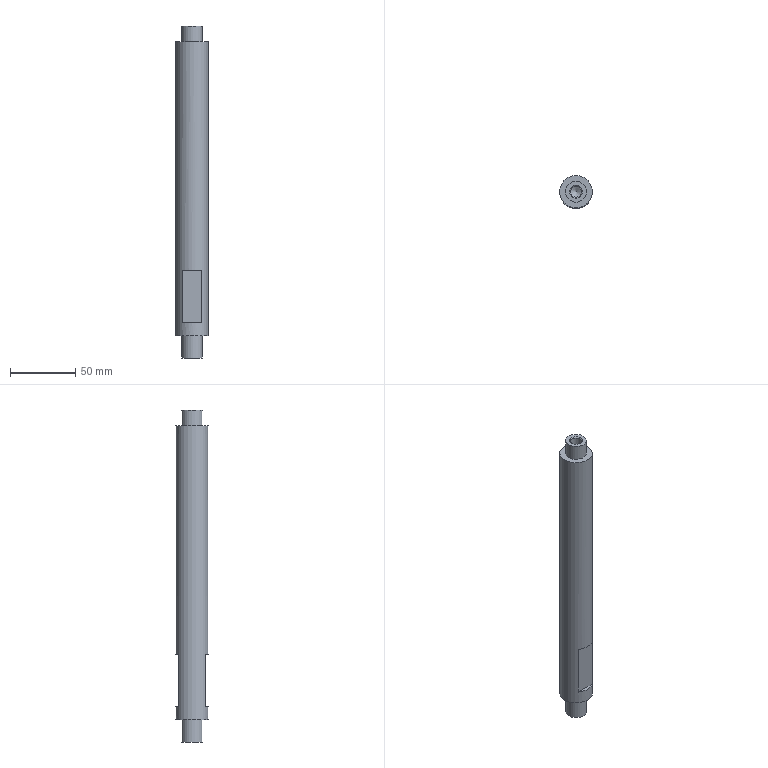Part | STEP file | YBQDJ-QD-2 | 1 solid | 19 faces | box 25 x 25 x 254 mm | volume 111454 mm3 | plane 10 | cylinder 5 | cone 4 | commonest cylinder face diameters 8.5 x2 16 x2 25 x1
STEP:
#1=CARTESIAN_POINT('',(0.,0.,0.));
#2=DIRECTION('',(0.,0.,1.));
#3=DIRECTION('',(1.,0.,0.));
#4=AXIS2_PLACEMENT_3D('',#1,#2,#3);
#5=CARTESIAN_POINT('',(-327.5,-310.,250.));
#6=VERTEX_POINT('',#5);
#7=CARTESIAN_POINT('',(-340.,-310.,250.));
#8=DIRECTION('',(0.,0.,1.));
#9=DIRECTION('',(1.,0.,0.));
#10=AXIS2_PLACEMENT_3D('',#7,#8,#9);
#11=CIRCLE('',#10,12.5);
#12=CARTESIAN_POINT('',(-340.,-310.,270.));
#13=DIRECTION('',(0.,0.,-1.));
#14=DIRECTION('',(-1.,0.,0.));
#15=AXIS2_PLACEMENT_3D('',#12,#13,#14);
#16=CYLINDRICAL_SURFACE('',#15,12.5);
#17=CARTESIAN_POINT('',(9.425,20.));
#18=DIRECTION('',(-1.,0.));
#19=VECTOR('',#18,1.);
#20=LINE('',#17,#19);
#21=(GEOMETRIC_REPRESENTATION_CONTEXT(2)PARAMETRIC_REPRESENTATION_CONTEXT()REPRESENTATION_CONTEXT('',''));
#22=DEFINITIONAL_REPRESENTATION('',(#20),#21);
#23=PCURVE('',#16,#22);
#24=CARTESIAN_POINT('',(-340.,-310.,250.));
#25=DIRECTION('',(0.,0.,1.));
#26=DIRECTION('',(1.,0.,0.));
#27=AXIS2_PLACEMENT_3D('',#24,#25,#26);
#28=PLANE('',#27);
#29=CARTESIAN_POINT('',(0.,0.));
#30=DIRECTION('',(1.,0.));
#31=AXIS2_PLACEMENT_2D('',#29,#30);
#32=CIRCLE('',#31,12.5);
#33=(GEOMETRIC_REPRESENTATION_CONTEXT(2)PARAMETRIC_REPRESENTATION_CONTEXT()REPRESENTATION_CONTEXT('',''));
#34=DEFINITIONAL_REPRESENTATION('',(#32),#33);
#35=PCURVE('',#28,#34);
#36=SURFACE_CURVE('',#11,(#23,#35),.PCURVE_S1.);
#37=EDGE_CURVE('',#6,#6,#36,.T.);
#38=ORIENTED_EDGE('',*,*,#37,.F.);
#39=CARTESIAN_POINT('',(-327.5,-310.,25.));
#40=VERTEX_POINT('',#39);
#41=CARTESIAN_POINT('',(-327.5,-310.,250.));
#42=CARTESIAN_POINT('',(-327.5,-310.,25.));
#43=B_SPLINE_CURVE_WITH_KNOTS('',1,(#41,#42),.UNSPECIFIED.,.F.,.F.,(2,2),(20.,245.),.PIECEWISE_BEZIER_KNOTS.);
#44=CARTESIAN_POINT('',(9.425,0.));
#45=DIRECTION('',(0.,1.));
#46=VECTOR('',#45,1.);
#47=LINE('',#44,#46);
#48=(GEOMETRIC_REPRESENTATION_CONTEXT(2)PARAMETRIC_REPRESENTATION_CONTEXT()REPRESENTATION_CONTEXT('',''));
#49=DEFINITIONAL_REPRESENTATION('',(#47),#48);
#50=PCURVE('',#16,#49);
#51=CARTESIAN_POINT('',(3.142,0.));
#52=DIRECTION('',(0.,1.));
#53=VECTOR('',#52,1.);
#54=LINE('',#51,#53);
#55=(GEOMETRIC_REPRESENTATION_CONTEXT(2)PARAMETRIC_REPRESENTATION_CONTEXT()REPRESENTATION_CONTEXT('',''));
#56=DEFINITIONAL_REPRESENTATION('',(#54),#55);
#57=PCURVE('',#16,#56);
#58=SEAM_CURVE('',#43,(#50,#57),.PCURVE_S1.);
#59=EDGE_CURVE('',#6,#40,#58,.T.);
#60=ORIENTED_EDGE('',*,*,#59,.T.);
#61=CARTESIAN_POINT('',(-340.,-310.,25.));
#62=DIRECTION('',(0.,0.,1.));
#63=DIRECTION('',(1.,0.,0.));
#64=AXIS2_PLACEMENT_3D('',#61,#62,#63);
#65=CIRCLE('',#64,12.5);
#66=CARTESIAN_POINT('',(9.425,245.));
#67=DIRECTION('',(-1.,0.));
#68=VECTOR('',#67,1.);
#69=LINE('',#66,#68);
#70=(GEOMETRIC_REPRESENTATION_CONTEXT(2)PARAMETRIC_REPRESENTATION_CONTEXT()REPRESENTATION_CONTEXT('',''));
#71=DEFINITIONAL_REPRESENTATION('',(#69),#70);
#72=PCURVE('',#16,#71);
#73=CARTESIAN_POINT('',(92.5,10.,25.));
#74=DIRECTION('',(0.,0.,1.));
#75=DIRECTION('',(1.,0.,0.));
#76=AXIS2_PLACEMENT_3D('',#73,#74,#75);
#77=PLANE('',#76);
#78=CARTESIAN_POINT('',(-432.5,-320.));
#79=DIRECTION('',(1.,0.));
#80=AXIS2_PLACEMENT_2D('',#78,#79);
#81=CIRCLE('',#80,12.5);
#82=(GEOMETRIC_REPRESENTATION_CONTEXT(2)PARAMETRIC_REPRESENTATION_CONTEXT()REPRESENTATION_CONTEXT('',''));
#83=DEFINITIONAL_REPRESENTATION('',(#81),#82);
#84=PCURVE('',#77,#83);
#85=SURFACE_CURVE('',#65,(#72,#84),.PCURVE_S1.);
#86=EDGE_CURVE('',#40,#40,#85,.T.);
#87=ORIENTED_EDGE('',*,*,#86,.T.);
#88=ORIENTED_EDGE('',*,*,#59,.F.);
#89=EDGE_LOOP('',(#38,#60,#87,#88));
#90=FACE_BOUND('',#89,.T.);
#91=CARTESIAN_POINT('',(-347.5,-300.,75.));
#92=VERTEX_POINT('',#91);
#93=CARTESIAN_POINT('',(-332.5,-300.,75.));
#94=VERTEX_POINT('',#93);
#95=CARTESIAN_POINT('',(-340.,-310.,75.));
#96=DIRECTION('',(0.,0.,-1.));
#97=DIRECTION('',(0.,1.,0.));
#98=AXIS2_PLACEMENT_3D('',#95,#96,#97);
#99=CIRCLE('',#98,12.5);
#100=CARTESIAN_POINT('',(1.571,195.));
#101=DIRECTION('',(1.,0.));
#102=VECTOR('',#101,1.);
#103=LINE('',#100,#102);
#104=(GEOMETRIC_REPRESENTATION_CONTEXT(2)PARAMETRIC_REPRESENTATION_CONTEXT()REPRESENTATION_CONTEXT('',''));
#105=DEFINITIONAL_REPRESENTATION('',(#103),#104);
#106=PCURVE('',#16,#105);
#107=CARTESIAN_POINT('',(-382.,-300.,75.));
#108=DIRECTION('',(0.,0.,-1.));
#109=DIRECTION('',(0.,1.,0.));
#110=AXIS2_PLACEMENT_3D('',#107,#108,#109);
#111=PLANE('',#110);
#112=CARTESIAN_POINT('',(-10.,42.));
#113=DIRECTION('',(1.,0.));
#114=AXIS2_PLACEMENT_2D('',#112,#113);
#115=CIRCLE('',#114,12.5);
#116=(GEOMETRIC_REPRESENTATION_CONTEXT(2)PARAMETRIC_REPRESENTATION_CONTEXT()REPRESENTATION_CONTEXT('',''));
#117=DEFINITIONAL_REPRESENTATION('',(#115),#116);
#118=PCURVE('',#111,#117);
#119=SURFACE_CURVE('',#99,(#106,#118),.PCURVE_S1.);
#120=EDGE_CURVE('',#92,#94,#119,.T.);
#121=ORIENTED_EDGE('',*,*,#120,.F.);
#122=CARTESIAN_POINT('',(-347.5,-300.,35.));
#123=VERTEX_POINT('',#122);
#124=CARTESIAN_POINT('',(-347.5,-300.,270.));
#125=DIRECTION('',(0.,0.,1.));
#126=VECTOR('',#125,1.);
#127=LINE('',#124,#126);
#128=CARTESIAN_POINT('',(7.21,0.));
#129=DIRECTION('',(0.,-1.));
#130=VECTOR('',#129,1.);
#131=LINE('',#128,#130);
#132=(GEOMETRIC_REPRESENTATION_CONTEXT(2)PARAMETRIC_REPRESENTATION_CONTEXT()REPRESENTATION_CONTEXT('',''));
#133=DEFINITIONAL_REPRESENTATION('',(#131),#132);
#134=PCURVE('',#16,#133);
#135=CARTESIAN_POINT('',(-382.,-300.,35.));
#136=DIRECTION('',(0.,1.,0.));
#137=DIRECTION('',(0.,0.,1.));
#138=AXIS2_PLACEMENT_3D('',#135,#136,#137);
#139=PLANE('',#138);
#140=CARTESIAN_POINT('',(235.,34.5));
#141=DIRECTION('',(1.,0.));
#142=VECTOR('',#141,1.);
#143=LINE('',#140,#142);
#144=(GEOMETRIC_REPRESENTATION_CONTEXT(2)PARAMETRIC_REPRESENTATION_CONTEXT()REPRESENTATION_CONTEXT('',''));
#145=DEFINITIONAL_REPRESENTATION('',(#143),#144);
#146=PCURVE('',#139,#145);
#147=SURFACE_CURVE('',#127,(#134,#146),.PCURVE_S1.);
#148=EDGE_CURVE('',#123,#92,#147,.T.);
#149=ORIENTED_EDGE('',*,*,#148,.F.);
#150=CARTESIAN_POINT('',(-332.5,-300.,35.));
#151=VERTEX_POINT('',#150);
#152=CARTESIAN_POINT('',(-340.,-310.,35.));
#153=DIRECTION('',(0.,0.,1.));
#154=DIRECTION('',(0.,-1.,0.));
#155=AXIS2_PLACEMENT_3D('',#152,#153,#154);
#156=CIRCLE('',#155,12.5);
#157=CARTESIAN_POINT('',(10.996,235.));
#158=DIRECTION('',(-1.,0.));
#159=VECTOR('',#158,1.);
#160=LINE('',#157,#159);
#161=(GEOMETRIC_REPRESENTATION_CONTEXT(2)PARAMETRIC_REPRESENTATION_CONTEXT()REPRESENTATION_CONTEXT('',''));
#162=DEFINITIONAL_REPRESENTATION('',(#160),#161);
#163=PCURVE('',#16,#162);
#164=CARTESIAN_POINT('',(-382.,-281.,35.));
#165=DIRECTION('',(0.,0.,1.));
#166=DIRECTION('',(0.,-1.,0.));
#167=AXIS2_PLACEMENT_3D('',#164,#165,#166);
#168=PLANE('',#167);
#169=CARTESIAN_POINT('',(29.,42.));
#170=DIRECTION('',(1.,0.));
#171=AXIS2_PLACEMENT_2D('',#169,#170);
#172=CIRCLE('',#171,12.5);
#173=(GEOMETRIC_REPRESENTATION_CONTEXT(2)PARAMETRIC_REPRESENTATION_CONTEXT()REPRESENTATION_CONTEXT('',''));
#174=DEFINITIONAL_REPRESENTATION('',(#172),#173);
#175=PCURVE('',#168,#174);
#176=SURFACE_CURVE('',#156,(#163,#175),.PCURVE_S1.);
#177=EDGE_CURVE('',#151,#123,#176,.T.);
#178=ORIENTED_EDGE('',*,*,#177,.F.);
#179=CARTESIAN_POINT('',(-332.5,-300.,270.));
#180=DIRECTION('',(0.,0.,-1.));
#181=VECTOR('',#180,1.);
#182=LINE('',#179,#181);
#183=CARTESIAN_POINT('',(8.497,0.));
#184=DIRECTION('',(0.,1.));
#185=VECTOR('',#184,1.);
#186=LINE('',#183,#185);
#187=(GEOMETRIC_REPRESENTATION_CONTEXT(2)PARAMETRIC_REPRESENTATION_CONTEXT()REPRESENTATION_CONTEXT('',''));
#188=DEFINITIONAL_REPRESENTATION('',(#186),#187);
#189=PCURVE('',#16,#188);
#190=CARTESIAN_POINT('',(235.,49.5));
#191=DIRECTION('',(-1.,0.));
#192=VECTOR('',#191,1.);
#193=LINE('',#190,#192);
#194=(GEOMETRIC_REPRESENTATION_CONTEXT(2)PARAMETRIC_REPRESENTATION_CONTEXT()REPRESENTATION_CONTEXT('',''));
#195=DEFINITIONAL_REPRESENTATION('',(#193),#194);
#196=PCURVE('',#139,#195);
#197=SURFACE_CURVE('',#182,(#189,#196),.PCURVE_S1.);
#198=EDGE_CURVE('',#94,#151,#197,.T.);
#199=ORIENTED_EDGE('',*,*,#198,.F.);
#200=EDGE_LOOP('',(#121,#149,#178,#199));
#201=FACE_BOUND('',#200,.T.);
#202=CARTESIAN_POINT('',(-332.5,-320.,75.));
#203=VERTEX_POINT('',#202);
#204=CARTESIAN_POINT('',(-347.5,-320.,75.));
#205=VERTEX_POINT('',#204);
#206=CARTESIAN_POINT('',(-340.,-310.,75.));
#207=DIRECTION('',(0.,0.,-1.));
#208=DIRECTION('',(0.,1.,0.));
#209=AXIS2_PLACEMENT_3D('',#206,#207,#208);
#210=CIRCLE('',#209,12.5);
#211=CARTESIAN_POINT('',(1.571,195.));
#212=DIRECTION('',(1.,0.));
#213=VECTOR('',#212,1.);
#214=LINE('',#211,#213);
#215=(GEOMETRIC_REPRESENTATION_CONTEXT(2)PARAMETRIC_REPRESENTATION_CONTEXT()REPRESENTATION_CONTEXT('',''));
#216=DEFINITIONAL_REPRESENTATION('',(#214),#215);
#217=PCURVE('',#16,#216);
#218=CARTESIAN_POINT('',(-382.,-339.,75.));
#219=DIRECTION('',(0.,0.,-1.));
#220=DIRECTION('',(0.,1.,0.));
#221=AXIS2_PLACEMENT_3D('',#218,#219,#220);
#222=PLANE('',#221);
#223=CARTESIAN_POINT('',(29.,42.));
#224=DIRECTION('',(1.,0.));
#225=AXIS2_PLACEMENT_2D('',#223,#224);
#226=CIRCLE('',#225,12.5);
#227=(GEOMETRIC_REPRESENTATION_CONTEXT(2)PARAMETRIC_REPRESENTATION_CONTEXT()REPRESENTATION_CONTEXT('',''));
#228=DEFINITIONAL_REPRESENTATION('',(#226),#227);
#229=PCURVE('',#222,#228);
#230=SURFACE_CURVE('',#210,(#217,#229),.PCURVE_S1.);
#231=EDGE_CURVE('',#203,#205,#230,.T.);
#232=ORIENTED_EDGE('',*,*,#231,.F.);
#233=CARTESIAN_POINT('',(-332.5,-320.,35.));
#234=VERTEX_POINT('',#233);
#235=CARTESIAN_POINT('',(-332.5,-320.,270.));
#236=DIRECTION('',(0.,0.,1.));
#237=VECTOR('',#236,1.);
#238=LINE('',#235,#237);
#239=CARTESIAN_POINT('',(4.069,0.));
#240=DIRECTION('',(0.,-1.));
#241=VECTOR('',#240,1.);
#242=LINE('',#239,#241);
#243=(GEOMETRIC_REPRESENTATION_CONTEXT(2)PARAMETRIC_REPRESENTATION_CONTEXT()REPRESENTATION_CONTEXT('',''));
#244=DEFINITIONAL_REPRESENTATION('',(#242),#243);
#245=PCURVE('',#16,#244);
#246=CARTESIAN_POINT('',(-382.,-320.,65.));
#247=DIRECTION('',(0.,-1.,0.));
#248=DIRECTION('',(0.,0.,-1.));
#249=AXIS2_PLACEMENT_3D('',#246,#247,#248);
#250=PLANE('',#249);
#251=CARTESIAN_POINT('',(-205.,49.5));
#252=DIRECTION('',(-1.,0.));
#253=VECTOR('',#252,1.);
#254=LINE('',#251,#253);
#255=(GEOMETRIC_REPRESENTATION_CONTEXT(2)PARAMETRIC_REPRESENTATION_CONTEXT()REPRESENTATION_CONTEXT('',''));
#256=DEFINITIONAL_REPRESENTATION('',(#254),#255);
#257=PCURVE('',#250,#256);
#258=SURFACE_CURVE('',#238,(#245,#257),.PCURVE_S1.);
#259=EDGE_CURVE('',#234,#203,#258,.T.);
#260=ORIENTED_EDGE('',*,*,#259,.F.);
#261=CARTESIAN_POINT('',(-347.5,-320.,35.));
#262=VERTEX_POINT('',#261);
#263=CARTESIAN_POINT('',(-340.,-310.,35.));
#264=DIRECTION('',(0.,0.,1.));
#265=DIRECTION('',(0.,-1.,0.));
#266=AXIS2_PLACEMENT_3D('',#263,#264,#265);
#267=CIRCLE('',#266,12.5);
#268=CARTESIAN_POINT('',(10.996,235.));
#269=DIRECTION('',(-1.,0.));
#270=VECTOR('',#269,1.);
#271=LINE('',#268,#270);
#272=(GEOMETRIC_REPRESENTATION_CONTEXT(2)PARAMETRIC_REPRESENTATION_CONTEXT()REPRESENTATION_CONTEXT('',''));
#273=DEFINITIONAL_REPRESENTATION('',(#271),#272);
#274=PCURVE('',#16,#273);
#275=CARTESIAN_POINT('',(-382.,-320.,35.));
#276=DIRECTION('',(0.,0.,1.));
#277=DIRECTION('',(0.,-1.,0.));
#278=AXIS2_PLACEMENT_3D('',#275,#276,#277);
#279=PLANE('',#278);
#280=CARTESIAN_POINT('',(-10.,42.));
#281=DIRECTION('',(1.,0.));
#282=AXIS2_PLACEMENT_2D('',#280,#281);
#283=CIRCLE('',#282,12.5);
#284=(GEOMETRIC_REPRESENTATION_CONTEXT(2)PARAMETRIC_REPRESENTATION_CONTEXT()REPRESENTATION_CONTEXT('',''));
#285=DEFINITIONAL_REPRESENTATION('',(#283),#284);
#286=PCURVE('',#279,#285);
#287=SURFACE_CURVE('',#267,(#274,#286),.PCURVE_S1.);
#288=EDGE_CURVE('',#262,#234,#287,.T.);
#289=ORIENTED_EDGE('',*,*,#288,.F.);
#290=CARTESIAN_POINT('',(-347.5,-320.,270.));
#291=DIRECTION('',(0.,0.,-1.));
#292=VECTOR('',#291,1.);
#293=LINE('',#290,#292);
#294=CARTESIAN_POINT('',(5.356,0.));
#295=DIRECTION('',(0.,1.));
#296=VECTOR('',#295,1.);
#297=LINE('',#294,#296);
#298=(GEOMETRIC_REPRESENTATION_CONTEXT(2)PARAMETRIC_REPRESENTATION_CONTEXT()REPRESENTATION_CONTEXT('',''));
#299=DEFINITIONAL_REPRESENTATION('',(#297),#298);
#300=PCURVE('',#16,#299);
#301=CARTESIAN_POINT('',(-205.,34.5));
#302=DIRECTION('',(1.,0.));
#303=VECTOR('',#302,1.);
#304=LINE('',#301,#303);
#305=(GEOMETRIC_REPRESENTATION_CONTEXT(2)PARAMETRIC_REPRESENTATION_CONTEXT()REPRESENTATION_CONTEXT('',''));
#306=DEFINITIONAL_REPRESENTATION('',(#304),#305);
#307=PCURVE('',#250,#306);
#308=SURFACE_CURVE('',#293,(#300,#307),.PCURVE_S1.);
#309=EDGE_CURVE('',#205,#262,#308,.T.);
#310=ORIENTED_EDGE('',*,*,#309,.F.);
#311=EDGE_LOOP('',(#232,#260,#289,#310));
#312=FACE_BOUND('',#311,.T.);
#313=ADVANCED_FACE('',(#90,#201,#312),#16,.T.);
#314=CARTESIAN_POINT('',(-332.,-310.,250.));
#315=VERTEX_POINT('',#314);
#316=CARTESIAN_POINT('',(-340.,-310.,250.));
#317=DIRECTION('',(0.,0.,1.));
#318=DIRECTION('',(1.,0.,0.));
#319=AXIS2_PLACEMENT_3D('',#316,#317,#318);
#320=CIRCLE('',#319,8.);
#321=CARTESIAN_POINT('',(0.,0.));
#322=DIRECTION('',(1.,0.));
#323=AXIS2_PLACEMENT_2D('',#321,#322);
#324=CIRCLE('',#323,8.);
#325=(GEOMETRIC_REPRESENTATION_CONTEXT(2)PARAMETRIC_REPRESENTATION_CONTEXT()REPRESENTATION_CONTEXT('',''));
#326=DEFINITIONAL_REPRESENTATION('',(#324),#325);
#327=PCURVE('',#28,#326);
#328=CARTESIAN_POINT('',(-340.,-310.,265.));
#329=DIRECTION('',(0.,0.,-1.));
#330=DIRECTION('',(-1.,0.,0.));
#331=AXIS2_PLACEMENT_3D('',#328,#329,#330);
#332=CYLINDRICAL_SURFACE('',#331,8.);
#333=CARTESIAN_POINT('',(9.425,15.));
#334=DIRECTION('',(-1.,0.));
#335=VECTOR('',#334,1.);
#336=LINE('',#333,#335);
#337=(GEOMETRIC_REPRESENTATION_CONTEXT(2)PARAMETRIC_REPRESENTATION_CONTEXT()REPRESENTATION_CONTEXT('',''));
#338=DEFINITIONAL_REPRESENTATION('',(#336),#337);
#339=PCURVE('',#332,#338);
#340=SURFACE_CURVE('',#320,(#327,#339),.PCURVE_S1.);
#341=EDGE_CURVE('',#315,#315,#340,.T.);
#342=ORIENTED_EDGE('',*,*,#341,.F.);
#343=EDGE_LOOP('',(#342));
#344=FACE_BOUND('',#343,.T.);
#345=ORIENTED_EDGE('',*,*,#37,.T.);
#346=EDGE_LOOP('',(#345));
#347=FACE_BOUND('',#346,.T.);
#348=ADVANCED_FACE('',(#344,#347),#28,.T.);
#349=CARTESIAN_POINT('',(-332.,-310.,25.));
#350=VERTEX_POINT('',#349);
#351=CARTESIAN_POINT('',(-340.,-310.,25.));
#352=DIRECTION('',(0.,0.,-1.));
#353=DIRECTION('',(1.,0.,0.));
#354=AXIS2_PLACEMENT_3D('',#351,#352,#353);
#355=CIRCLE('',#354,8.);
#356=CARTESIAN_POINT('',(-424.5,-320.));
#357=CARTESIAN_POINT('',(-424.5,-333.856));
#358=CARTESIAN_POINT('',(-436.5,-326.928));
#359=CARTESIAN_POINT('',(-448.5,-320.));
#360=CARTESIAN_POINT('',(-436.5,-313.072));
#361=CARTESIAN_POINT('',(-424.5,-306.144));
#362=CARTESIAN_POINT('',(-424.5,-320.));
#363=(BOUNDED_CURVE()B_SPLINE_CURVE(2,(#356,#357,#358,#359,#360,#361,#362),.UNSPECIFIED.,.T.,.F.)B_SPLINE_CURVE_WITH_KNOTS((1,2,2,2,2,1),(-2.094,0.,2.094,4.189,6.283,8.378),.UNSPECIFIED.)CURVE()GEOMETRIC_REPRESENTATION_ITEM()RATIONAL_B_SPLINE_CURVE((1.,0.5,1.,0.5,1.,0.5,1.))REPRESENTATION_ITEM(''));
#364=(GEOMETRIC_REPRESENTATION_CONTEXT(2)PARAMETRIC_REPRESENTATION_CONTEXT()REPRESENTATION_CONTEXT('',''));
#365=DEFINITIONAL_REPRESENTATION('',(#363),#364);
#366=PCURVE('',#77,#365);
#367=CARTESIAN_POINT('',(-340.,-310.,8.));
#368=DIRECTION('',(0.,0.,1.));
#369=DIRECTION('',(1.,0.,0.));
#370=AXIS2_PLACEMENT_3D('',#367,#368,#369);
#371=CYLINDRICAL_SURFACE('',#370,8.);
#372=CARTESIAN_POINT('',(6.283,17.));
#373=DIRECTION('',(-1.,0.));
#374=VECTOR('',#373,1.);
#375=LINE('',#372,#374);
#376=(GEOMETRIC_REPRESENTATION_CONTEXT(2)PARAMETRIC_REPRESENTATION_CONTEXT()REPRESENTATION_CONTEXT('',''));
#377=DEFINITIONAL_REPRESENTATION('',(#375),#376);
#378=PCURVE('',#371,#377);
#379=SURFACE_CURVE('',#355,(#366,#378),.PCURVE_S1.);
#380=EDGE_CURVE('',#350,#350,#379,.T.);
#381=ORIENTED_EDGE('',*,*,#380,.F.);
#382=EDGE_LOOP('',(#381));
#383=FACE_BOUND('',#382,.T.);
#384=ORIENTED_EDGE('',*,*,#86,.F.);
#385=EDGE_LOOP('',(#384));
#386=FACE_BOUND('',#385,.T.);
#387=ADVANCED_FACE('',(#383,#386),#77,.F.);
#388=CARTESIAN_POINT('',(-332.,-310.,262.));
#389=VERTEX_POINT('',#388);
#390=CARTESIAN_POINT('',(-340.,-310.,262.));
#391=DIRECTION('',(0.,0.,1.));
#392=DIRECTION('',(1.,0.,0.));
#393=AXIS2_PLACEMENT_3D('',#390,#391,#392);
#394=CIRCLE('',#393,8.);
#395=CARTESIAN_POINT('',(9.425,3.));
#396=DIRECTION('',(-1.,0.));
#397=VECTOR('',#396,1.);
#398=LINE('',#395,#397);
#399=(GEOMETRIC_REPRESENTATION_CONTEXT(2)PARAMETRIC_REPRESENTATION_CONTEXT()REPRESENTATION_CONTEXT('',''));
#400=DEFINITIONAL_REPRESENTATION('',(#398),#399);
#401=PCURVE('',#332,#400);
#402=CARTESIAN_POINT('',(-340.,-310.,262.));
#403=DIRECTION('',(0.,0.,1.));
#404=DIRECTION('',(1.,0.,0.));
#405=AXIS2_PLACEMENT_3D('',#402,#403,#404);
#406=PLANE('',#405);
#407=CARTESIAN_POINT('',(0.,0.));
#408=DIRECTION('',(1.,0.));
#409=AXIS2_PLACEMENT_2D('',#407,#408);
#410=CIRCLE('',#409,8.);
#411=(GEOMETRIC_REPRESENTATION_CONTEXT(2)PARAMETRIC_REPRESENTATION_CONTEXT()REPRESENTATION_CONTEXT('',''));
#412=DEFINITIONAL_REPRESENTATION('',(#410),#411);
#413=PCURVE('',#406,#412);
#414=SURFACE_CURVE('',#394,(#401,#413),.PCURVE_S1.);
#415=EDGE_CURVE('',#389,#389,#414,.T.);
#416=ORIENTED_EDGE('',*,*,#415,.F.);
#417=CARTESIAN_POINT('',(-332.,-310.,262.));
#418=CARTESIAN_POINT('',(-332.,-310.,250.));
#419=B_SPLINE_CURVE_WITH_KNOTS('',1,(#417,#418),.UNSPECIFIED.,.F.,.F.,(2,2),(3.,15.),.PIECEWISE_BEZIER_KNOTS.);
#420=CARTESIAN_POINT('',(9.425,0.));
#421=DIRECTION('',(0.,1.));
#422=VECTOR('',#421,1.);
#423=LINE('',#420,#422);
#424=(GEOMETRIC_REPRESENTATION_CONTEXT(2)PARAMETRIC_REPRESENTATION_CONTEXT()REPRESENTATION_CONTEXT('',''));
#425=DEFINITIONAL_REPRESENTATION('',(#423),#424);
#426=PCURVE('',#332,#425);
#427=CARTESIAN_POINT('',(3.142,0.));
#428=DIRECTION('',(0.,1.));
#429=VECTOR('',#428,1.);
#430=LINE('',#427,#429);
#431=(GEOMETRIC_REPRESENTATION_CONTEXT(2)PARAMETRIC_REPRESENTATION_CONTEXT()REPRESENTATION_CONTEXT('',''));
#432=DEFINITIONAL_REPRESENTATION('',(#430),#431);
#433=PCURVE('',#332,#432);
#434=SEAM_CURVE('',#419,(#426,#433),.PCURVE_S1.);
#435=EDGE_CURVE('',#389,#315,#434,.T.);
#436=ORIENTED_EDGE('',*,*,#435,.T.);
#437=ORIENTED_EDGE('',*,*,#341,.T.);
#438=ORIENTED_EDGE('',*,*,#435,.F.);
#439=EDGE_LOOP('',(#416,#436,#437,#438));
#440=FACE_BOUND('',#439,.T.);
#441=ADVANCED_FACE('',(#440),#332,.T.);
#442=CARTESIAN_POINT('',(-335.,-310.,262.));
#443=VERTEX_POINT('',#442);
#444=CARTESIAN_POINT('',(-340.,-310.,262.));
#445=DIRECTION('',(0.,0.,-1.));
#446=DIRECTION('',(1.,0.,0.));
#447=AXIS2_PLACEMENT_3D('',#444,#445,#446);
#448=CIRCLE('',#447,5.);
#449=CARTESIAN_POINT('',(5.,0.));
#450=CARTESIAN_POINT('',(5.,-8.66));
#451=CARTESIAN_POINT('',(-2.5,-4.33));
#452=CARTESIAN_POINT('',(-10.,0.));
#453=CARTESIAN_POINT('',(-2.5,4.33));
#454=CARTESIAN_POINT('',(5.,8.66));
#455=CARTESIAN_POINT('',(5.,0.));
#456=(BOUNDED_CURVE()B_SPLINE_CURVE(2,(#449,#450,#451,#452,#453,#454,#455),.UNSPECIFIED.,.T.,.F.)B_SPLINE_CURVE_WITH_KNOTS((1,2,2,2,2,1),(-2.094,0.,2.094,4.189,6.283,8.378),.UNSPECIFIED.)CURVE()GEOMETRIC_REPRESENTATION_ITEM()RATIONAL_B_SPLINE_CURVE((1.,0.5,1.,0.5,1.,0.5,1.))REPRESENTATION_ITEM(''));
#457=(GEOMETRIC_REPRESENTATION_CONTEXT(2)PARAMETRIC_REPRESENTATION_CONTEXT()REPRESENTATION_CONTEXT('',''));
#458=DEFINITIONAL_REPRESENTATION('',(#456),#457);
#459=PCURVE('',#406,#458);
#460=CARTESIAN_POINT('',(-340.,-310.,262.));
#461=DIRECTION('',(0.,0.,1.));
#462=DIRECTION('',(1.,0.,0.));
#463=AXIS2_PLACEMENT_3D('',#460,#461,#462);
#464=CONICAL_SURFACE('',#463,5.,0.7854);
#465=CARTESIAN_POINT('',(6.283,0.));
#466=DIRECTION('',(-1.,0.));
#467=VECTOR('',#466,1.);
#468=LINE('',#465,#467);
#469=(GEOMETRIC_REPRESENTATION_CONTEXT(2)PARAMETRIC_REPRESENTATION_CONTEXT()REPRESENTATION_CONTEXT('',''));
#470=DEFINITIONAL_REPRESENTATION('',(#468),#469);
#471=PCURVE('',#464,#470);
#472=SURFACE_CURVE('',#448,(#459,#471),.PCURVE_S1.);
#473=EDGE_CURVE('',#443,#443,#472,.T.);
#474=ORIENTED_EDGE('',*,*,#473,.T.);
#475=EDGE_LOOP('',(#474));
#476=FACE_BOUND('',#475,.T.);
#477=ORIENTED_EDGE('',*,*,#415,.T.);
#478=EDGE_LOOP('',(#477));
#479=FACE_BOUND('',#478,.T.);
#480=ADVANCED_FACE('',(#476,#479),#406,.T.);
#481=CARTESIAN_POINT('',(-335.75,-310.,240.));
#482=VERTEX_POINT('',#481);
#483=CARTESIAN_POINT('',(-344.25,-310.,240.));
#484=VERTEX_POINT('',#483);
#485=CARTESIAN_POINT('',(-340.,-310.,240.));
#486=DIRECTION('',(0.,0.,1.));
#487=DIRECTION('',(-1.,0.,0.));
#488=AXIS2_PLACEMENT_3D('',#485,#486,#487);
#489=CIRCLE('',#488,4.25);
#490=CARTESIAN_POINT('',(-340.,-310.,240.));
#491=DIRECTION('',(0.,0.,1.));
#492=DIRECTION('',(1.,0.,0.));
#493=AXIS2_PLACEMENT_3D('',#490,#491,#492);
#494=CONICAL_SURFACE('',#493,4.25,1.03);
#495=CARTESIAN_POINT('',(-3.142,0.));
#496=DIRECTION('',(1.,0.));
#497=VECTOR('',#496,1.);
#498=LINE('',#495,#497);
#499=(GEOMETRIC_REPRESENTATION_CONTEXT(2)PARAMETRIC_REPRESENTATION_CONTEXT()REPRESENTATION_CONTEXT('',''));
#500=DEFINITIONAL_REPRESENTATION('',(#498),#499);
#501=PCURVE('',#494,#500);
#502=CARTESIAN_POINT('',(-340.,-310.,265.));
#503=DIRECTION('',(0.,0.,-1.));
#504=DIRECTION('',(-1.,0.,0.));
#505=AXIS2_PLACEMENT_3D('',#502,#503,#504);
#506=CYLINDRICAL_SURFACE('',#505,4.25);
#507=CARTESIAN_POINT('',(12.566,25.));
#508=DIRECTION('',(-1.,0.));
#509=VECTOR('',#508,1.);
#510=LINE('',#507,#509);
#511=(GEOMETRIC_REPRESENTATION_CONTEXT(2)PARAMETRIC_REPRESENTATION_CONTEXT()REPRESENTATION_CONTEXT('',''));
#512=DEFINITIONAL_REPRESENTATION('',(#510),#511);
#513=PCURVE('',#506,#512);
#514=SURFACE_CURVE('',#489,(#501,#513),.PCURVE_S1.);
#515=EDGE_CURVE('',#482,#484,#514,.T.);
#516=ORIENTED_EDGE('',*,*,#515,.F.);
#517=CARTESIAN_POINT('',(-340.,-310.,237.446));
#518=VERTEX_POINT('',#517);
#519=CARTESIAN_POINT('',(-340.,-310.,237.446));
#520=CARTESIAN_POINT('',(-335.75,-310.,240.));
#521=B_SPLINE_CURVE_WITH_KNOTS('',1,(#519,#520),.UNSPECIFIED.,.F.,.F.,(2,2),(-4.958,0.),.PIECEWISE_BEZIER_KNOTS.);
#522=CARTESIAN_POINT('',(0.,0.));
#523=DIRECTION('',(0.,1.));
#524=VECTOR('',#523,1.);
#525=LINE('',#522,#524);
#526=(GEOMETRIC_REPRESENTATION_CONTEXT(2)PARAMETRIC_REPRESENTATION_CONTEXT()REPRESENTATION_CONTEXT('',''));
#527=DEFINITIONAL_REPRESENTATION('',(#525),#526);
#528=PCURVE('',#494,#527);
#529=CARTESIAN_POINT('',(6.283,0.));
#530=DIRECTION('',(0.,1.));
#531=VECTOR('',#530,1.);
#532=LINE('',#529,#531);
#533=(GEOMETRIC_REPRESENTATION_CONTEXT(2)PARAMETRIC_REPRESENTATION_CONTEXT()REPRESENTATION_CONTEXT('',''));
#534=DEFINITIONAL_REPRESENTATION('',(#532),#533);
#535=PCURVE('',#494,#534);
#536=SEAM_CURVE('',#521,(#528,#535),.PCURVE_S1.);
#537=EDGE_CURVE('',#518,#482,#536,.T.);
#538=ORIENTED_EDGE('',*,*,#537,.F.);
#539=ORIENTED_EDGE('',*,*,#537,.T.);
#540=CARTESIAN_POINT('',(-340.,-310.,240.));
#541=DIRECTION('',(0.,0.,1.));
#542=DIRECTION('',(-1.,0.,0.));
#543=AXIS2_PLACEMENT_3D('',#540,#541,#542);
#544=CIRCLE('',#543,4.25);
#545=CARTESIAN_POINT('',(3.142,0.));
#546=DIRECTION('',(1.,0.));
#547=VECTOR('',#546,1.);
#548=LINE('',#545,#547);
#549=(GEOMETRIC_REPRESENTATION_CONTEXT(2)PARAMETRIC_REPRESENTATION_CONTEXT()REPRESENTATION_CONTEXT('',''));
#550=DEFINITIONAL_REPRESENTATION('',(#548),#549);
#551=PCURVE('',#494,#550);
#552=CARTESIAN_POINT('',(6.283,25.));
#553=DIRECTION('',(-1.,0.));
#554=VECTOR('',#553,1.);
#555=LINE('',#552,#554);
#556=(GEOMETRIC_REPRESENTATION_CONTEXT(2)PARAMETRIC_REPRESENTATION_CONTEXT()REPRESENTATION_CONTEXT('',''));
#557=DEFINITIONAL_REPRESENTATION('',(#555),#556);
#558=PCURVE('',#506,#557);
#559=SURFACE_CURVE('',#544,(#551,#558),.PCURVE_S1.);
#560=EDGE_CURVE('',#484,#482,#559,.T.);
#561=ORIENTED_EDGE('',*,*,#560,.F.);
#562=EDGE_LOOP('',(#516,#538,#539,#561));
#563=FACE_BOUND('',#562,.F.);
#564=ADVANCED_FACE('',(#563),#494,.F.);
#565=CARTESIAN_POINT('',(-335.75,-310.,261.25));
#566=VERTEX_POINT('',#565);
#567=CARTESIAN_POINT('',(-340.,-310.,261.25));
#568=DIRECTION('',(0.,0.,1.));
#569=DIRECTION('',(1.,0.,0.));
#570=AXIS2_PLACEMENT_3D('',#567,#568,#569);
#571=CIRCLE('',#570,4.25);
#572=CARTESIAN_POINT('',(9.425,3.75));
#573=DIRECTION('',(-1.,0.));
#574=VECTOR('',#573,1.);
#575=LINE('',#572,#574);
#576=(GEOMETRIC_REPRESENTATION_CONTEXT(2)PARAMETRIC_REPRESENTATION_CONTEXT()REPRESENTATION_CONTEXT('',''));
#577=DEFINITIONAL_REPRESENTATION('',(#575),#576);
#578=PCURVE('',#506,#577);
#579=CARTESIAN_POINT('',(0.,-0.75));
#580=DIRECTION('',(1.,0.));
#581=VECTOR('',#580,1.);
#582=LINE('',#579,#581);
#583=(GEOMETRIC_REPRESENTATION_CONTEXT(2)PARAMETRIC_REPRESENTATION_CONTEXT()REPRESENTATION_CONTEXT('',''));
#584=DEFINITIONAL_REPRESENTATION('',(#582),#583);
#585=PCURVE('',#464,#584);
#586=SURFACE_CURVE('',#571,(#578,#585),.PCURVE_S1.);
#587=EDGE_CURVE('',#566,#566,#586,.T.);
#588=ORIENTED_EDGE('',*,*,#587,.F.);
#589=CARTESIAN_POINT('',(-335.75,-310.,261.25));
#590=CARTESIAN_POINT('',(-335.75,-310.,240.));
#591=B_SPLINE_CURVE_WITH_KNOTS('',1,(#589,#590),.UNSPECIFIED.,.F.,.F.,(2,2),(3.75,25.),.PIECEWISE_BEZIER_KNOTS.);
#592=CARTESIAN_POINT('',(9.425,0.));
#593=DIRECTION('',(0.,1.));
#594=VECTOR('',#593,1.);
#595=LINE('',#592,#594);
#596=(GEOMETRIC_REPRESENTATION_CONTEXT(2)PARAMETRIC_REPRESENTATION_CONTEXT()REPRESENTATION_CONTEXT('',''));
#597=DEFINITIONAL_REPRESENTATION('',(#595),#596);
#598=PCURVE('',#506,#597);
#599=CARTESIAN_POINT('',(3.142,0.));
#600=DIRECTION('',(0.,1.));
#601=VECTOR('',#600,1.);
#602=LINE('',#599,#601);
#603=(GEOMETRIC_REPRESENTATION_CONTEXT(2)PARAMETRIC_REPRESENTATION_CONTEXT()REPRESENTATION_CONTEXT('',''));
#604=DEFINITIONAL_REPRESENTATION('',(#602),#603);
#605=PCURVE('',#506,#604);
#606=SEAM_CURVE('',#591,(#598,#605),.PCURVE_S1.);
#607=EDGE_CURVE('',#566,#482,#606,.T.);
#608=ORIENTED_EDGE('',*,*,#607,.T.);
#609=ORIENTED_EDGE('',*,*,#515,.T.);
#610=ORIENTED_EDGE('',*,*,#560,.T.);
#611=ORIENTED_EDGE('',*,*,#607,.F.);
#612=EDGE_LOOP('',(#588,#608,#609,#610,#611));
#613=FACE_BOUND('',#612,.F.);
#614=ADVANCED_FACE('',(#613),#506,.F.);
#615=ORIENTED_EDGE('',*,*,#587,.T.);
#616=CARTESIAN_POINT('',(-335.75,-310.,261.25));
#617=CARTESIAN_POINT('',(-335.,-310.,262.));
#618=B_SPLINE_CURVE_WITH_KNOTS('',1,(#616,#617),.UNSPECIFIED.,.F.,.F.,(2,2),(-1.061,0.),.PIECEWISE_BEZIER_KNOTS.);
#619=CARTESIAN_POINT('',(6.283,0.));
#620=DIRECTION('',(0.,1.));
#621=VECTOR('',#620,1.);
#622=LINE('',#619,#621);
#623=(GEOMETRIC_REPRESENTATION_CONTEXT(2)PARAMETRIC_REPRESENTATION_CONTEXT()REPRESENTATION_CONTEXT('',''));
#624=DEFINITIONAL_REPRESENTATION('',(#622),#623);
#625=PCURVE('',#464,#624);
#626=CARTESIAN_POINT('',(0.,0.));
#627=DIRECTION('',(0.,1.));
#628=VECTOR('',#627,1.);
#629=LINE('',#626,#628);
#630=(GEOMETRIC_REPRESENTATION_CONTEXT(2)PARAMETRIC_REPRESENTATION_CONTEXT()REPRESENTATION_CONTEXT('',''));
#631=DEFINITIONAL_REPRESENTATION('',(#629),#630);
#632=PCURVE('',#464,#631);
#633=SEAM_CURVE('',#618,(#625,#632),.PCURVE_S1.);
#634=EDGE_CURVE('',#566,#443,#633,.T.);
#635=ORIENTED_EDGE('',*,*,#634,.T.);
#636=ORIENTED_EDGE('',*,*,#473,.T.);
#637=ORIENTED_EDGE('',*,*,#634,.F.);
#638=EDGE_LOOP('',(#615,#635,#636,#637));
#639=FACE_BOUND('',#638,.F.);
#640=ADVANCED_FACE('',(#639),#464,.F.);
#641=CARTESIAN_POINT('',(-332.,-310.,8.));
#642=VERTEX_POINT('',#641);
#643=CARTESIAN_POINT('',(-348.,-310.,8.));
#644=VERTEX_POINT('',#643);
#645=CARTESIAN_POINT('',(-340.,-310.,8.));
#646=DIRECTION('',(0.,0.,-1.));
#647=DIRECTION('',(-1.,0.,0.));
#648=AXIS2_PLACEMENT_3D('',#645,#646,#647);
#649=CIRCLE('',#648,8.);
#650=CARTESIAN_POINT('',(9.425,0.));
#651=DIRECTION('',(-1.,0.));
#652=VECTOR('',#651,1.);
#653=LINE('',#650,#652);
#654=(GEOMETRIC_REPRESENTATION_CONTEXT(2)PARAMETRIC_REPRESENTATION_CONTEXT()REPRESENTATION_CONTEXT('',''));
#655=DEFINITIONAL_REPRESENTATION('',(#653),#654);
#656=PCURVE('',#371,#655);
#657=CARTESIAN_POINT('',(-340.,-310.,8.));
#658=DIRECTION('',(0.,0.,-1.));
#659=DIRECTION('',(-1.,0.,0.));
#660=AXIS2_PLACEMENT_3D('',#657,#658,#659);
#661=PLANE('',#660);
#662=CARTESIAN_POINT('',(0.,0.));
#663=DIRECTION('',(1.,0.));
#664=AXIS2_PLACEMENT_2D('',#662,#663);
#665=CIRCLE('',#664,8.);
#666=(GEOMETRIC_REPRESENTATION_CONTEXT(2)PARAMETRIC_REPRESENTATION_CONTEXT()REPRESENTATION_CONTEXT('',''));
#667=DEFINITIONAL_REPRESENTATION('',(#665),#666);
#668=PCURVE('',#661,#667);
#669=SURFACE_CURVE('',#649,(#656,#668),.PCURVE_S1.);
#670=EDGE_CURVE('',#642,#644,#669,.T.);
#671=ORIENTED_EDGE('',*,*,#670,.F.);
#672=CARTESIAN_POINT('',(-332.,-310.,8.));
#673=CARTESIAN_POINT('',(-332.,-310.,25.));
#674=B_SPLINE_CURVE_WITH_KNOTS('',1,(#672,#673),.UNSPECIFIED.,.F.,.F.,(2,2),(0.,17.),.PIECEWISE_BEZIER_KNOTS.);
#675=CARTESIAN_POINT('',(6.283,0.));
#676=DIRECTION('',(0.,1.));
#677=VECTOR('',#676,1.);
#678=LINE('',#675,#677);
#679=(GEOMETRIC_REPRESENTATION_CONTEXT(2)PARAMETRIC_REPRESENTATION_CONTEXT()REPRESENTATION_CONTEXT('',''));
#680=DEFINITIONAL_REPRESENTATION('',(#678),#679);
#681=PCURVE('',#371,#680);
#682=CARTESIAN_POINT('',(0.,0.));
#683=DIRECTION('',(0.,1.));
#684=VECTOR('',#683,1.);
#685=LINE('',#682,#684);
#686=(GEOMETRIC_REPRESENTATION_CONTEXT(2)PARAMETRIC_REPRESENTATION_CONTEXT()REPRESENTATION_CONTEXT('',''));
#687=DEFINITIONAL_REPRESENTATION('',(#685),#686);
#688=PCURVE('',#371,#687);
#689=SEAM_CURVE('',#674,(#681,#688),.PCURVE_S1.);
#690=EDGE_CURVE('',#642,#350,#689,.T.);
#691=ORIENTED_EDGE('',*,*,#690,.T.);
#692=ORIENTED_EDGE('',*,*,#380,.T.);
#693=ORIENTED_EDGE('',*,*,#690,.F.);
#694=CARTESIAN_POINT('',(-340.,-310.,8.));
#695=DIRECTION('',(0.,0.,-1.));
#696=DIRECTION('',(-1.,0.,0.));
#697=AXIS2_PLACEMENT_3D('',#694,#695,#696);
#698=CIRCLE('',#697,8.);
#699=CARTESIAN_POINT('',(3.142,0.));
#700=DIRECTION('',(-1.,0.));
#701=VECTOR('',#700,1.);
#702=LINE('',#699,#701);
#703=(GEOMETRIC_REPRESENTATION_CONTEXT(2)PARAMETRIC_REPRESENTATION_CONTEXT()REPRESENTATION_CONTEXT('',''));
#704=DEFINITIONAL_REPRESENTATION('',(#702),#703);
#705=PCURVE('',#371,#704);
#706=CARTESIAN_POINT('',(0.,0.));
#707=DIRECTION('',(1.,0.));
#708=AXIS2_PLACEMENT_2D('',#706,#707);
#709=CIRCLE('',#708,8.);
#710=(GEOMETRIC_REPRESENTATION_CONTEXT(2)PARAMETRIC_REPRESENTATION_CONTEXT()REPRESENTATION_CONTEXT('',''));
#711=DEFINITIONAL_REPRESENTATION('',(#709),#710);
#712=PCURVE('',#661,#711);
#713=SURFACE_CURVE('',#698,(#705,#712),.PCURVE_S1.);
#714=EDGE_CURVE('',#644,#642,#713,.T.);
#715=ORIENTED_EDGE('',*,*,#714,.F.);
#716=EDGE_LOOP('',(#671,#691,#692,#693,#715));
#717=FACE_BOUND('',#716,.T.);
#718=ADVANCED_FACE('',(#717),#371,.T.);
#719=CARTESIAN_POINT('',(-345.,-310.,8.));
#720=VERTEX_POINT('',#719);
#721=CARTESIAN_POINT('',(-340.,-310.,8.));
#722=DIRECTION('',(0.,0.,1.));
#723=DIRECTION('',(-1.,0.,0.));
#724=AXIS2_PLACEMENT_3D('',#721,#722,#723);
#725=CIRCLE('',#724,5.);
#726=CARTESIAN_POINT('',(5.,0.));
#727=CARTESIAN_POINT('',(5.,-8.66));
#728=CARTESIAN_POINT('',(-2.5,-4.33));
#729=CARTESIAN_POINT('',(-10.,0.));
#730=CARTESIAN_POINT('',(-2.5,4.33));
#731=CARTESIAN_POINT('',(5.,8.66));
#732=CARTESIAN_POINT('',(5.,0.));
#733=(BOUNDED_CURVE()B_SPLINE_CURVE(2,(#726,#727,#728,#729,#730,#731,#732),.UNSPECIFIED.,.T.,.F.)B_SPLINE_CURVE_WITH_KNOTS((1,2,2,2,2,1),(-2.094,0.,2.094,4.189,6.283,8.378),.UNSPECIFIED.)CURVE()GEOMETRIC_REPRESENTATION_ITEM()RATIONAL_B_SPLINE_CURVE((1.,0.5,1.,0.5,1.,0.5,1.))REPRESENTATION_ITEM(''));
#734=(GEOMETRIC_REPRESENTATION_CONTEXT(2)PARAMETRIC_REPRESENTATION_CONTEXT()REPRESENTATION_CONTEXT('',''));
#735=DEFINITIONAL_REPRESENTATION('',(#733),#734);
#736=PCURVE('',#661,#735);
#737=CARTESIAN_POINT('',(-340.,-310.,8.));
#738=DIRECTION('',(0.,0.,-1.));
#739=DIRECTION('',(-1.,0.,0.));
#740=AXIS2_PLACEMENT_3D('',#737,#738,#739);
#741=CONICAL_SURFACE('',#740,5.,0.7854);
#742=CARTESIAN_POINT('',(6.283,0.));
#743=DIRECTION('',(-1.,0.));
#744=VECTOR('',#743,1.);
#745=LINE('',#742,#744);
#746=(GEOMETRIC_REPRESENTATION_CONTEXT(2)PARAMETRIC_REPRESENTATION_CONTEXT()REPRESENTATION_CONTEXT('',''));
#747=DEFINITIONAL_REPRESENTATION('',(#745),#746);
#748=PCURVE('',#741,#747);
#749=SURFACE_CURVE('',#725,(#736,#748),.PCURVE_S1.);
#750=EDGE_CURVE('',#720,#720,#749,.T.);
#751=ORIENTED_EDGE('',*,*,#750,.T.);
#752=EDGE_LOOP('',(#751));
#753=FACE_BOUND('',#752,.T.);
#754=ORIENTED_EDGE('',*,*,#714,.T.);
#755=ORIENTED_EDGE('',*,*,#670,.T.);
#756=EDGE_LOOP('',(#754,#755));
#757=FACE_BOUND('',#756,.T.);
#758=ADVANCED_FACE('',(#753,#757),#661,.T.);
#759=CARTESIAN_POINT('',(-344.25,-310.,33.));
#760=VERTEX_POINT('',#759);
#761=CARTESIAN_POINT('',(-335.75,-310.,33.));
#762=VERTEX_POINT('',#761);
#763=CARTESIAN_POINT('',(-340.,-310.,33.));
#764=DIRECTION('',(0.,0.,-1.));
#765=DIRECTION('',(1.,0.,0.));
#766=AXIS2_PLACEMENT_3D('',#763,#764,#765);
#767=CIRCLE('',#766,4.25);
#768=CARTESIAN_POINT('',(-340.,-310.,33.));
#769=DIRECTION('',(0.,0.,-1.));
#770=DIRECTION('',(-1.,0.,0.));
#771=AXIS2_PLACEMENT_3D('',#768,#769,#770);
#772=CONICAL_SURFACE('',#771,4.25,1.03);
#773=CARTESIAN_POINT('',(-3.142,0.));
#774=DIRECTION('',(1.,0.));
#775=VECTOR('',#774,1.);
#776=LINE('',#773,#775);
#777=(GEOMETRIC_REPRESENTATION_CONTEXT(2)PARAMETRIC_REPRESENTATION_CONTEXT()REPRESENTATION_CONTEXT('',''));
#778=DEFINITIONAL_REPRESENTATION('',(#776),#777);
#779=PCURVE('',#772,#778);
#780=CARTESIAN_POINT('',(-340.,-310.,8.));
#781=DIRECTION('',(0.,0.,1.));
#782=DIRECTION('',(1.,0.,0.));
#783=AXIS2_PLACEMENT_3D('',#780,#781,#782);
#784=CYLINDRICAL_SURFACE('',#783,4.25);
#785=CARTESIAN_POINT('',(12.566,25.));
#786=DIRECTION('',(-1.,0.));
#787=VECTOR('',#786,1.);
#788=LINE('',#785,#787);
#789=(GEOMETRIC_REPRESENTATION_CONTEXT(2)PARAMETRIC_REPRESENTATION_CONTEXT()REPRESENTATION_CONTEXT('',''));
#790=DEFINITIONAL_REPRESENTATION('',(#788),#789);
#791=PCURVE('',#784,#790);
#792=SURFACE_CURVE('',#767,(#779,#791),.PCURVE_S1.);
#793=EDGE_CURVE('',#760,#762,#792,.T.);
#794=ORIENTED_EDGE('',*,*,#793,.F.);
#795=CARTESIAN_POINT('',(-340.,-310.,35.554));
#796=VERTEX_POINT('',#795);
#797=CARTESIAN_POINT('',(-340.,-310.,35.554));
#798=CARTESIAN_POINT('',(-344.25,-310.,33.));
#799=B_SPLINE_CURVE_WITH_KNOTS('',1,(#797,#798),.UNSPECIFIED.,.F.,.F.,(2,2),(-4.958,0.),.PIECEWISE_BEZIER_KNOTS.);
#800=CARTESIAN_POINT('',(0.,0.));
#801=DIRECTION('',(0.,1.));
#802=VECTOR('',#801,1.);
#803=LINE('',#800,#802);
#804=(GEOMETRIC_REPRESENTATION_CONTEXT(2)PARAMETRIC_REPRESENTATION_CONTEXT()REPRESENTATION_CONTEXT('',''));
#805=DEFINITIONAL_REPRESENTATION('',(#803),#804);
#806=PCURVE('',#772,#805);
#807=CARTESIAN_POINT('',(6.283,0.));
#808=DIRECTION('',(0.,1.));
#809=VECTOR('',#808,1.);
#810=LINE('',#807,#809);
#811=(GEOMETRIC_REPRESENTATION_CONTEXT(2)PARAMETRIC_REPRESENTATION_CONTEXT()REPRESENTATION_CONTEXT('',''));
#812=DEFINITIONAL_REPRESENTATION('',(#810),#811);
#813=PCURVE('',#772,#812);
#814=SEAM_CURVE('',#799,(#806,#813),.PCURVE_S1.);
#815=EDGE_CURVE('',#796,#760,#814,.T.);
#816=ORIENTED_EDGE('',*,*,#815,.F.);
#817=ORIENTED_EDGE('',*,*,#815,.T.);
#818=CARTESIAN_POINT('',(-340.,-310.,33.));
#819=DIRECTION('',(0.,0.,-1.));
#820=DIRECTION('',(1.,0.,0.));
#821=AXIS2_PLACEMENT_3D('',#818,#819,#820);
#822=CIRCLE('',#821,4.25);
#823=CARTESIAN_POINT('',(3.142,0.));
#824=DIRECTION('',(1.,0.));
#825=VECTOR('',#824,1.);
#826=LINE('',#823,#825);
#827=(GEOMETRIC_REPRESENTATION_CONTEXT(2)PARAMETRIC_REPRESENTATION_CONTEXT()REPRESENTATION_CONTEXT('',''));
#828=DEFINITIONAL_REPRESENTATION('',(#826),#827);
#829=PCURVE('',#772,#828);
#830=CARTESIAN_POINT('',(6.283,25.));
#831=DIRECTION('',(-1.,0.));
#832=VECTOR('',#831,1.);
#833=LINE('',#830,#832);
#834=(GEOMETRIC_REPRESENTATION_CONTEXT(2)PARAMETRIC_REPRESENTATION_CONTEXT()REPRESENTATION_CONTEXT('',''));
#835=DEFINITIONAL_REPRESENTATION('',(#833),#834);
#836=PCURVE('',#784,#835);
#837=SURFACE_CURVE('',#822,(#829,#836),.PCURVE_S1.);
#838=EDGE_CURVE('',#762,#760,#837,.T.);
#839=ORIENTED_EDGE('',*,*,#838,.F.);
#840=EDGE_LOOP('',(#794,#816,#817,#839));
#841=FACE_BOUND('',#840,.F.);
#842=ADVANCED_FACE('',(#841),#772,.F.);
#843=CARTESIAN_POINT('',(-344.25,-310.,8.75));
#844=VERTEX_POINT('',#843);
#845=CARTESIAN_POINT('',(-340.,-310.,8.75));
#846=DIRECTION('',(0.,0.,-1.));
#847=DIRECTION('',(-1.,0.,0.));
#848=AXIS2_PLACEMENT_3D('',#845,#846,#847);
#849=CIRCLE('',#848,4.25);
#850=CARTESIAN_POINT('',(9.425,0.75));
#851=DIRECTION('',(-1.,0.));
#852=VECTOR('',#851,1.);
#853=LINE('',#850,#852);
#854=(GEOMETRIC_REPRESENTATION_CONTEXT(2)PARAMETRIC_REPRESENTATION_CONTEXT()REPRESENTATION_CONTEXT('',''));
#855=DEFINITIONAL_REPRESENTATION('',(#853),#854);
#856=PCURVE('',#784,#855);
#857=CARTESIAN_POINT('',(0.,-0.75));
#858=DIRECTION('',(1.,0.));
#859=VECTOR('',#858,1.);
#860=LINE('',#857,#859);
#861=(GEOMETRIC_REPRESENTATION_CONTEXT(2)PARAMETRIC_REPRESENTATION_CONTEXT()REPRESENTATION_CONTEXT('',''));
#862=DEFINITIONAL_REPRESENTATION('',(#860),#861);
#863=PCURVE('',#741,#862);
#864=SURFACE_CURVE('',#849,(#856,#863),.PCURVE_S1.);
#865=EDGE_CURVE('',#844,#844,#864,.T.);
#866=ORIENTED_EDGE('',*,*,#865,.F.);
#867=CARTESIAN_POINT('',(-344.25,-310.,8.75));
#868=CARTESIAN_POINT('',(-344.25,-310.,33.));
#869=B_SPLINE_CURVE_WITH_KNOTS('',1,(#867,#868),.UNSPECIFIED.,.F.,.F.,(2,2),(0.75,25.),.PIECEWISE_BEZIER_KNOTS.);
#870=CARTESIAN_POINT('',(9.425,0.));
#871=DIRECTION('',(0.,1.));
#872=VECTOR('',#871,1.);
#873=LINE('',#870,#872);
#874=(GEOMETRIC_REPRESENTATION_CONTEXT(2)PARAMETRIC_REPRESENTATION_CONTEXT()REPRESENTATION_CONTEXT('',''));
#875=DEFINITIONAL_REPRESENTATION('',(#873),#874);
#876=PCURVE('',#784,#875);
#877=CARTESIAN_POINT('',(3.142,0.));
#878=DIRECTION('',(0.,1.));
#879=VECTOR('',#878,1.);
#880=LINE('',#877,#879);
#881=(GEOMETRIC_REPRESENTATION_CONTEXT(2)PARAMETRIC_REPRESENTATION_CONTEXT()REPRESENTATION_CONTEXT('',''));
#882=DEFINITIONAL_REPRESENTATION('',(#880),#881);
#883=PCURVE('',#784,#882);
#884=SEAM_CURVE('',#869,(#876,#883),.PCURVE_S1.);
#885=EDGE_CURVE('',#844,#760,#884,.T.);
#886=ORIENTED_EDGE('',*,*,#885,.T.);
#887=ORIENTED_EDGE('',*,*,#793,.T.);
#888=ORIENTED_EDGE('',*,*,#838,.T.);
#889=ORIENTED_EDGE('',*,*,#885,.F.);
#890=EDGE_LOOP('',(#866,#886,#887,#888,#889));
#891=FACE_BOUND('',#890,.F.);
#892=ADVANCED_FACE('',(#891),#784,.F.);
#893=ORIENTED_EDGE('',*,*,#865,.T.);
#894=CARTESIAN_POINT('',(-344.25,-310.,8.75));
#895=CARTESIAN_POINT('',(-345.,-310.,8.));
#896=B_SPLINE_CURVE_WITH_KNOTS('',1,(#894,#895),.UNSPECIFIED.,.F.,.F.,(2,2),(-1.061,0.),.PIECEWISE_BEZIER_KNOTS.);
#897=CARTESIAN_POINT('',(6.283,0.));
#898=DIRECTION('',(0.,1.));
#899=VECTOR('',#898,1.);
#900=LINE('',#897,#899);
#901=(GEOMETRIC_REPRESENTATION_CONTEXT(2)PARAMETRIC_REPRESENTATION_CONTEXT()REPRESENTATION_CONTEXT('',''));
#902=DEFINITIONAL_REPRESENTATION('',(#900),#901);
#903=PCURVE('',#741,#902);
#904=CARTESIAN_POINT('',(0.,0.));
#905=DIRECTION('',(0.,1.));
#906=VECTOR('',#905,1.);
#907=LINE('',#904,#906);
#908=(GEOMETRIC_REPRESENTATION_CONTEXT(2)PARAMETRIC_REPRESENTATION_CONTEXT()REPRESENTATION_CONTEXT('',''));
#909=DEFINITIONAL_REPRESENTATION('',(#907),#908);
#910=PCURVE('',#741,#909);
#911=SEAM_CURVE('',#896,(#903,#910),.PCURVE_S1.);
#912=EDGE_CURVE('',#844,#720,#911,.T.);
#913=ORIENTED_EDGE('',*,*,#912,.T.);
#914=ORIENTED_EDGE('',*,*,#750,.T.);
#915=ORIENTED_EDGE('',*,*,#912,.F.);
#916=EDGE_LOOP('',(#893,#913,#914,#915));
#917=FACE_BOUND('',#916,.F.);
#918=ADVANCED_FACE('',(#917),#741,.F.);
#919=ORIENTED_EDGE('',*,*,#198,.T.);
#920=CARTESIAN_POINT('',(-382.,-300.,35.));
#921=DIRECTION('',(-1.,0.,0.));
#922=VECTOR('',#921,1.);
#923=LINE('',#920,#922);
#924=CARTESIAN_POINT('',(0.,0.));
#925=DIRECTION('',(0.,-1.));
#926=VECTOR('',#925,1.);
#927=LINE('',#924,#926);
#928=(GEOMETRIC_REPRESENTATION_CONTEXT(2)PARAMETRIC_REPRESENTATION_CONTEXT()REPRESENTATION_CONTEXT('',''));
#929=DEFINITIONAL_REPRESENTATION('',(#927),#928);
#930=PCURVE('',#139,#929);
#931=CARTESIAN_POINT('',(19.,0.));
#932=DIRECTION('',(0.,-1.));
#933=VECTOR('',#932,1.);
#934=LINE('',#931,#933);
#935=(GEOMETRIC_REPRESENTATION_CONTEXT(2)PARAMETRIC_REPRESENTATION_CONTEXT()REPRESENTATION_CONTEXT('',''));
#936=DEFINITIONAL_REPRESENTATION('',(#934),#935);
#937=PCURVE('',#168,#936);
#938=SURFACE_CURVE('',#923,(#930,#937),.PCURVE_S1.);
#939=EDGE_CURVE('',#151,#123,#938,.T.);
#940=ORIENTED_EDGE('',*,*,#939,.T.);
#941=ORIENTED_EDGE('',*,*,#148,.T.);
#942=CARTESIAN_POINT('',(-382.,-300.,75.));
#943=DIRECTION('',(-1.,0.,0.));
#944=VECTOR('',#943,1.);
#945=LINE('',#942,#944);
#946=CARTESIAN_POINT('',(40.,0.));
#947=DIRECTION('',(0.,-1.));
#948=VECTOR('',#947,1.);
#949=LINE('',#946,#948);
#950=(GEOMETRIC_REPRESENTATION_CONTEXT(2)PARAMETRIC_REPRESENTATION_CONTEXT()REPRESENTATION_CONTEXT('',''));
#951=DEFINITIONAL_REPRESENTATION('',(#949),#950);
#952=PCURVE('',#139,#951);
#953=CARTESIAN_POINT('',(0.,0.));
#954=DIRECTION('',(0.,-1.));
#955=VECTOR('',#954,1.);
#956=LINE('',#953,#955);
#957=(GEOMETRIC_REPRESENTATION_CONTEXT(2)PARAMETRIC_REPRESENTATION_CONTEXT()REPRESENTATION_CONTEXT('',''));
#958=DEFINITIONAL_REPRESENTATION('',(#956),#957);
#959=PCURVE('',#111,#958);
#960=SURFACE_CURVE('',#945,(#952,#959),.PCURVE_S1.);
#961=EDGE_CURVE('',#94,#92,#960,.T.);
#962=ORIENTED_EDGE('',*,*,#961,.F.);
#963=EDGE_LOOP('',(#919,#940,#941,#962));
#964=FACE_BOUND('',#963,.T.);
#965=ADVANCED_FACE('',(#964),#139,.T.);
#966=ORIENTED_EDGE('',*,*,#120,.T.);
#967=ORIENTED_EDGE('',*,*,#961,.T.);
#968=EDGE_LOOP('',(#966,#967));
#969=FACE_BOUND('',#968,.T.);
#970=ADVANCED_FACE('',(#969),#111,.T.);
#971=ORIENTED_EDGE('',*,*,#177,.T.);
#972=ORIENTED_EDGE('',*,*,#939,.F.);
#973=EDGE_LOOP('',(#971,#972));
#974=FACE_BOUND('',#973,.T.);
#975=ADVANCED_FACE('',(#974),#168,.T.);
#976=ORIENTED_EDGE('',*,*,#231,.T.);
#977=CARTESIAN_POINT('',(-382.,-320.,75.));
#978=DIRECTION('',(-1.,0.,0.));
#979=VECTOR('',#978,1.);
#980=LINE('',#977,#979);
#981=CARTESIAN_POINT('',(19.,0.));
#982=DIRECTION('',(0.,-1.));
#983=VECTOR('',#982,1.);
#984=LINE('',#981,#983);
#985=(GEOMETRIC_REPRESENTATION_CONTEXT(2)PARAMETRIC_REPRESENTATION_CONTEXT()REPRESENTATION_CONTEXT('',''));
#986=DEFINITIONAL_REPRESENTATION('',(#984),#985);
#987=PCURVE('',#222,#986);
#988=CARTESIAN_POINT('',(-10.,0.));
#989=DIRECTION('',(0.,-1.));
#990=VECTOR('',#989,1.);
#991=LINE('',#988,#990);
#992=(GEOMETRIC_REPRESENTATION_CONTEXT(2)PARAMETRIC_REPRESENTATION_CONTEXT()REPRESENTATION_CONTEXT('',''));
#993=DEFINITIONAL_REPRESENTATION('',(#991),#992);
#994=PCURVE('',#250,#993);
#995=SURFACE_CURVE('',#980,(#987,#994),.PCURVE_S1.);
#996=EDGE_CURVE('',#203,#205,#995,.T.);
#997=ORIENTED_EDGE('',*,*,#996,.F.);
#998=EDGE_LOOP('',(#976,#997));
#999=FACE_BOUND('',#998,.T.);
#1000=ADVANCED_FACE('',(#999),#222,.T.);
#1001=ORIENTED_EDGE('',*,*,#309,.T.);
#1002=CARTESIAN_POINT('',(-382.,-320.,35.));
#1003=DIRECTION('',(-1.,0.,0.));
#1004=VECTOR('',#1003,1.);
#1005=LINE('',#1002,#1004);
#1006=CARTESIAN_POINT('',(30.,0.));
#1007=DIRECTION('',(0.,-1.));
#1008=VECTOR('',#1007,1.);
#1009=LINE('',#1006,#1008);
#1010=(GEOMETRIC_REPRESENTATION_CONTEXT(2)PARAMETRIC_REPRESENTATION_CONTEXT()REPRESENTATION_CONTEXT('',''));
#1011=DEFINITIONAL_REPRESENTATION('',(#1009),#1010);
#1012=PCURVE('',#250,#1011);
#1013=CARTESIAN_POINT('',(0.,0.));
#1014=DIRECTION('',(0.,-1.));
#1015=VECTOR('',#1014,1.);
#1016=LINE('',#1013,#1015);
#1017=(GEOMETRIC_REPRESENTATION_CONTEXT(2)PARAMETRIC_REPRESENTATION_CONTEXT()REPRESENTATION_CONTEXT('',''));
#1018=DEFINITIONAL_REPRESENTATION('',(#1016),#1017);
#1019=PCURVE('',#279,#1018);
#1020=SURFACE_CURVE('',#1005,(#1012,#1019),.PCURVE_S1.);
#1021=EDGE_CURVE('',#234,#262,#1020,.T.);
#1022=ORIENTED_EDGE('',*,*,#1021,.F.);
#1023=ORIENTED_EDGE('',*,*,#259,.T.);
#1024=ORIENTED_EDGE('',*,*,#996,.T.);
#1025=EDGE_LOOP('',(#1001,#1022,#1023,#1024));
#1026=FACE_BOUND('',#1025,.T.);
#1027=ADVANCED_FACE('',(#1026),#250,.T.);
#1028=ORIENTED_EDGE('',*,*,#288,.T.);
#1029=ORIENTED_EDGE('',*,*,#1021,.T.);
#1030=EDGE_LOOP('',(#1028,#1029));
#1031=FACE_BOUND('',#1030,.T.);
#1032=ADVANCED_FACE('',(#1031),#279,.T.);
#1033=CLOSED_SHELL('',(#313,#348,#387,#441,#480,#564,#614,#640,#718,#758,#842,#892,#918,#965,#970,#975,#1000,#1027,#1032));
#1034=MANIFOLD_SOLID_BREP('',#1033);
#1035=(LENGTH_UNIT()NAMED_UNIT(*)SI_UNIT(.MILLI.,.METRE.));
#1036=UNCERTAINTY_MEASURE_WITH_UNIT(LENGTH_MEASURE(0.000005),#1035,'','');
#1037=(NAMED_UNIT(*)PLANE_ANGLE_UNIT()SI_UNIT($,.RADIAN.));
#1038=(NAMED_UNIT(*)SI_UNIT($,.STERADIAN.)SOLID_ANGLE_UNIT());
#1039=(GEOMETRIC_REPRESENTATION_CONTEXT(3)GLOBAL_UNCERTAINTY_ASSIGNED_CONTEXT((#1036))GLOBAL_UNIT_ASSIGNED_CONTEXT((#1035,#1037,#1038))REPRESENTATION_CONTEXT('',''));
#1040=ADVANCED_BREP_SHAPE_REPRESENTATION('',(#4,#1034),#1039);